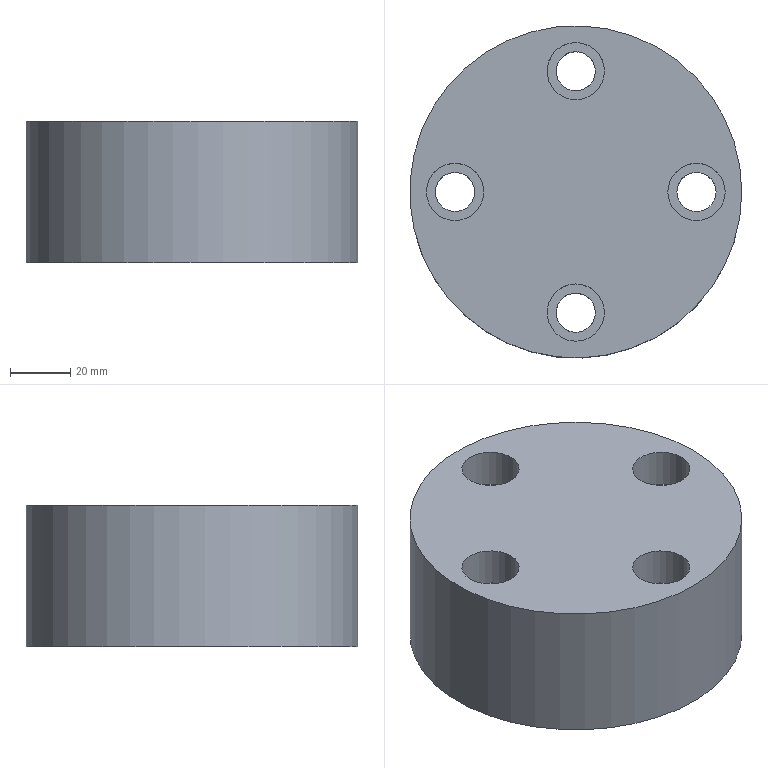NC program | NX | posted with a generic post | part box 110 x 110 x 47 mm
Whole program:
N10 G17 G21 G94 G90
(DRILLING , TOOL : ZXZ)
N12 T01 M6
N14 G54
N16 G17 G0 G90 X0. Y40. S3500 M3
N18 G43 Z30. H1
N20 G94 G81 G98 Z-1. F250. R3.
N22 X-40. Y0.
N24 X0. Y-40.
N26 X40. Y0.
N28 G80
N30 G0 X40. Y0. Z30.
N32 M5
(DRILLING_COPY_COPY , TOOL : 13.0ZT)
N34 T03 M6
N36 G54
N38 G17 G0 G90 X0. Y40. S500 M3
N40 G43 Z30. H3
N42 G94 G83 G98 Z-52.406 F150. Q3. R3.
N44 X-40. Y0.
N46 X0. Y-40.
N48 X40. Y0.
N50 G80
N52 G0 X40. Y0. Z30.
N54 M5
(HOLE_MILLING , TOOL : D10)
N56 T10 M6
N58 G54
N60 G17 G0 G90 X0. Y40. S3000 M3
N62 G43 Z30. H10
N64 Z0.5
N66 G94 G3 X2.25 Y37.75 R2.25 F2200.
N68 X4.5 Y40. R2.25
N70 X4.5 Y40. Z0.28 I-4.5 J0.
N72 X4.5 Y40. Z0.06 I-4.5 J0.
N74 X4.5 Y40. Z-0.16 I-4.5 J0.
N76 X4.5 Y40. Z-0.38 I-4.5 J0.
N78 X4.5 Y40. Z-0.6 I-4.5 J0.
N80 X4.5 Y40. Z-0.82 I-4.5 J0.
N82 X4.5 Y40. Z-1.04 I-4.5 J0.
N84 X4.5 Y40. Z-1.26 I-4.5 J0.
N86 X4.5 Y40. Z-1.48 I-4.5 J0.
N88 X4.5 Y40. Z-1.7 I-4.5 J0.
N90 X4.5 Y40. Z-1.92 I-4.5 J0.
N92 X4.5 Y40. Z-2.14 I-4.5 J0.
N94 X4.5 Y40. Z-2.36 I-4.5 J0.
N96 X4.5 Y40. Z-2.58 I-4.5 J0.
N98 X4.5 Y40. Z-2.8 I-4.5 J0.
N100 X4.5 Y40. Z-3.02 I-4.5 J0.
N102 X4.5 Y40. Z-3.24 I-4.5 J0.
N104 X4.5 Y40. Z-3.46 I-4.5 J0.
N106 X4.5 Y40. Z-3.68 I-4.5 J0.
N108 X4.5 Y40. Z-3.9 I-4.5 J0.
N110 X4.5 Y40. Z-4.12 I-4.5 J0.
N112 X4.5 Y40. Z-4.34 I-4.5 J0.
N114 X4.5 Y40. Z-4.56 I-4.5 J0.
N116 X4.5 Y40. Z-4.78 I-4.5 J0.
N118 X4.5 Y40. Z-5. I-4.5 J0.
N120 X4.5 Y40. Z-5.22 I-4.5 J0.
N122 X4.5 Y40. Z-5.44 I-4.5 J0.
N124 X4.5 Y40. Z-5.66 I-4.5 J0.
N126 X4.5 Y40. Z-5.88 I-4.5 J0.
N128 X4.5 Y40. Z-6.1 I-4.5 J0.
N130 X4.5 Y40. Z-6.32 I-4.5 J0.
N132 X4.5 Y40. Z-6.54 I-4.5 J0.
N134 X4.5 Y40. Z-6.76 I-4.5 J0.
N136 X4.5 Y40. Z-6.98 I-4.5 J0.
N138 X4.5 Y40. Z-7.2 I-4.5 J0.
N140 X4.5 Y40. Z-7.42 I-4.5 J0.
N142 X4.5 Y40. Z-7.64 I-4.5 J0.
N144 X4.5 Y40. Z-7.86 I-4.5 J0.
N146 X4.5 Y40. Z-8.08 I-4.5 J0.
N148 X4.5 Y40. Z-8.3 I-4.5 J0.
N150 X4.5 Y40. Z-8.52 I-4.5 J0.
N152 X4.5 Y40. Z-8.74 I-4.5 J0.
N154 X4.5 Y40. Z-8.96 I-4.5 J0.
N156 X4.5 Y40. Z-9.18 I-4.5 J0.
N158 X4.5 Y40. Z-9.4 I-4.5 J0.
N160 X4.5 Y40. Z-9.62 I-4.5 J0.
N162 X4.5 Y40. Z-9.84 I-4.5 J0.
N164 X4.5 Y40. Z-10.06 I-4.5 J0.
N166 X4.5 Y40. Z-10.28 I-4.5 J0.
N168 X4.5 Y40. Z-10.5 I-4.5 J0.
N170 X4.5 Y40. Z-10.72 I-4.5 J0.
N172 X4.5 Y40. Z-10.94 I-4.5 J0.
N174 X4.5 Y40. Z-11.16 I-4.5 J0.
N176 X4.5 Y40. Z-11.38 I-4.5 J0.
N178 X4.5 Y40. Z-11.6 I-4.5 J0.
N180 X4.5 Y40. Z-11.82 I-4.5 J0.
N182 X4.5 Y40. Z-12.04 I-4.5 J0.
N184 X4.5 Y40. Z-12.26 I-4.5 J0.
N186 X4.5 Y40. Z-12.48 I-4.5 J0.
N188 X4.5 Y40. Z-12.7 I-4.5 J0.
N190 X4.5 Y40. Z-12.92 I-4.5 J0.
N192 X-2.947 Y43.401 Z-13. R4.5
N194 X-3.401 Y37.053 R4.5
N196 X-2.947 Y43.401 R-4.5
N198 X-3.174 Y40.227 R2.25
N200 X0. Y40. R2.25
N202 G0 Z30.
N204 X-40. Y0.
N206 Z0.5
N208 G3 X-37.75 Y-2.25 R2.25
N210 X-35.5 Y0. R2.25
N212 X-35.5 Y0. Z0.28 I-4.5 J0.
N214 X-35.5 Y0. Z0.06 I-4.5 J0.
N216 X-35.5 Y0. Z-0.16 I-4.5 J0.
N218 X-35.5 Y0. Z-0.38 I-4.5 J0.
N220 X-35.5 Y0. Z-0.6 I-4.5 J0.
N222 X-35.5 Y0. Z-0.82 I-4.5 J0.
N224 X-35.5 Y0. Z-1.04 I-4.5 J0.
N226 X-35.5 Y0. Z-1.26 I-4.5 J0.
N228 X-35.5 Y0. Z-1.48 I-4.5 J0.
N230 X-35.5 Y0. Z-1.7 I-4.5 J0.
N232 X-35.5 Y0. Z-1.92 I-4.5 J0.
N234 X-35.5 Y0. Z-2.14 I-4.5 J0.
N236 X-35.5 Y0. Z-2.36 I-4.5 J0.
N238 X-35.5 Y0. Z-2.58 I-4.5 J0.
N240 X-35.5 Y0. Z-2.8 I-4.5 J0.
N242 X-35.5 Y0. Z-3.02 I-4.5 J0.
N244 X-35.5 Y0. Z-3.24 I-4.5 J0.
N246 X-35.5 Y0. Z-3.46 I-4.5 J0.
N248 X-35.5 Y0. Z-3.68 I-4.5 J0.
N250 X-35.5 Y0. Z-3.9 I-4.5 J0.
N252 X-35.5 Y0. Z-4.12 I-4.5 J0.
N254 X-35.5 Y0. Z-4.34 I-4.5 J0.
N256 X-35.5 Y0. Z-4.56 I-4.5 J0.
N258 X-35.5 Y0. Z-4.78 I-4.5 J0.
N260 X-35.5 Y0. Z-5. I-4.5 J0.
N262 X-35.5 Y0. Z-5.22 I-4.5 J0.
N264 X-35.5 Y0. Z-5.44 I-4.5 J0.
N266 X-35.5 Y0. Z-5.66 I-4.5 J0.
N268 X-35.5 Y0. Z-5.88 I-4.5 J0.
N270 X-35.5 Y0. Z-6.1 I-4.5 J0.
N272 X-35.5 Y0. Z-6.32 I-4.5 J0.
N274 X-35.5 Y0. Z-6.54 I-4.5 J0.
N276 X-35.5 Y0. Z-6.76 I-4.5 J0.
N278 X-35.5 Y0. Z-6.98 I-4.5 J0.
N280 X-35.5 Y0. Z-7.2 I-4.5 J0.
N282 X-35.5 Y0. Z-7.42 I-4.5 J0.
N284 X-35.5 Y0. Z-7.64 I-4.5 J0.
N286 X-35.5 Y0. Z-7.86 I-4.5 J0.
N288 X-35.5 Y0. Z-8.08 I-4.5 J0.
N290 X-35.5 Y0. Z-8.3 I-4.5 J0.
N292 X-35.5 Y0. Z-8.52 I-4.5 J0.
N294 X-35.5 Y0. Z-8.74 I-4.5 J0.
N296 X-35.5 Y0. Z-8.96 I-4.5 J0.
N298 X-35.5 Y0. Z-9.18 I-4.5 J0.
N300 X-35.5 Y0. Z-9.4 I-4.5 J0.
N302 X-35.5 Y0. Z-9.62 I-4.5 J0.
N304 X-35.5 Y0. Z-9.84 I-4.5 J0.
N306 X-35.5 Y0. Z-10.06 I-4.5 J0.
N308 X-35.5 Y0. Z-10.28 I-4.5 J0.
N310 X-35.5 Y0. Z-10.5 I-4.5 J0.
N312 X-35.5 Y0. Z-10.72 I-4.5 J0.
N314 X-35.5 Y0. Z-10.94 I-4.5 J0.
N316 X-35.5 Y0. Z-11.16 I-4.5 J0.
N318 X-35.5 Y0. Z-11.38 I-4.5 J0.
N320 X-35.5 Y0. Z-11.6 I-4.5 J0.
N322 X-35.5 Y0. Z-11.82 I-4.5 J0.
N324 X-35.5 Y0. Z-12.04 I-4.5 J0.
N326 X-35.5 Y0. Z-12.26 I-4.5 J0.
N328 X-35.5 Y0. Z-12.48 I-4.5 J0.
N330 X-35.5 Y0. Z-12.7 I-4.5 J0.
N332 X-35.5 Y0. Z-12.92 I-4.5 J0.
N334 X-42.947 Y3.401 Z-13. R4.5
N336 X-43.401 Y-2.947 R4.5
N338 X-42.947 Y3.401 R-4.5
N340 X-43.174 Y0.227 R2.25
N342 X-40. Y0. R2.25
N344 G0 Z30.
N346 X0. Y-40.
N348 Z0.5
N350 G3 X2.25 Y-42.25 R2.25
N352 X4.5 Y-40. R2.25
N354 X4.5 Y-40. Z0.28 I-4.5 J0.
N356 X4.5 Y-40. Z0.06 I-4.5 J0.
N358 X4.5 Y-40. Z-0.16 I-4.5 J0.
N360 X4.5 Y-40. Z-0.38 I-4.5 J0.
N362 X4.5 Y-40. Z-0.6 I-4.5 J0.
N364 X4.5 Y-40. Z-0.82 I-4.5 J0.
N366 X4.5 Y-40. Z-1.04 I-4.5 J0.
N368 X4.5 Y-40. Z-1.26 I-4.5 J0.
N370 X4.5 Y-40. Z-1.48 I-4.5 J0.
N372 X4.5 Y-40. Z-1.7 I-4.5 J0.
N374 X4.5 Y-40. Z-1.92 I-4.5 J0.
N376 X4.5 Y-40. Z-2.14 I-4.5 J0.
N378 X4.5 Y-40. Z-2.36 I-4.5 J0.
N380 X4.5 Y-40. Z-2.58 I-4.5 J0.
N382 X4.5 Y-40. Z-2.8 I-4.5 J0.
N384 X4.5 Y-40. Z-3.02 I-4.5 J0.
N386 X4.5 Y-40. Z-3.24 I-4.5 J0.
N388 X4.5 Y-40. Z-3.46 I-4.5 J0.
N390 X4.5 Y-40. Z-3.68 I-4.5 J0.
N392 X4.5 Y-40. Z-3.9 I-4.5 J0.
N394 X4.5 Y-40. Z-4.12 I-4.5 J0.
N396 X4.5 Y-40. Z-4.34 I-4.5 J0.
N398 X4.5 Y-40. Z-4.56 I-4.5 J0.
N400 X4.5 Y-40. Z-4.78 I-4.5 J0.
N402 X4.5 Y-40. Z-5. I-4.5 J0.
N404 X4.5 Y-40. Z-5.22 I-4.5 J0.
N406 X4.5 Y-40. Z-5.44 I-4.5 J0.
N408 X4.5 Y-40. Z-5.66 I-4.5 J0.
N410 X4.5 Y-40. Z-5.88 I-4.5 J0.
N412 X4.5 Y-40. Z-6.1 I-4.5 J0.
N414 X4.5 Y-40. Z-6.32 I-4.5 J0.
N416 X4.5 Y-40. Z-6.54 I-4.5 J0.
N418 X4.5 Y-40. Z-6.76 I-4.5 J0.
N420 X4.5 Y-40. Z-6.98 I-4.5 J0.
N422 X4.5 Y-40. Z-7.2 I-4.5 J0.
N424 X4.5 Y-40. Z-7.42 I-4.5 J0.
N426 X4.5 Y-40. Z-7.64 I-4.5 J0.
N428 X4.5 Y-40. Z-7.86 I-4.5 J0.
N430 X4.5 Y-40. Z-8.08 I-4.5 J0.
N432 X4.5 Y-40. Z-8.3 I-4.5 J0.
N434 X4.5 Y-40. Z-8.52 I-4.5 J0.
N436 X4.5 Y-40. Z-8.74 I-4.5 J0.
N438 X4.5 Y-40. Z-8.96 I-4.5 J0.
N440 X4.5 Y-40. Z-9.18 I-4.5 J0.
N442 X4.5 Y-40. Z-9.4 I-4.5 J0.
N444 X4.5 Y-40. Z-9.62 I-4.5 J0.
N446 X4.5 Y-40. Z-9.84 I-4.5 J0.
N448 X4.5 Y-40. Z-10.06 I-4.5 J0.
N450 X4.5 Y-40. Z-10.28 I-4.5 J0.
N452 X4.5 Y-40. Z-10.5 I-4.5 J0.
N454 X4.5 Y-40. Z-10.72 I-4.5 J0.
N456 X4.5 Y-40. Z-10.94 I-4.5 J0.
N458 X4.5 Y-40. Z-11.16 I-4.5 J0.
N460 X4.5 Y-40. Z-11.38 I-4.5 J0.
N462 X4.5 Y-40. Z-11.6 I-4.5 J0.
N464 X4.5 Y-40. Z-11.82 I-4.5 J0.
N466 X4.5 Y-40. Z-12.04 I-4.5 J0.
N468 X4.5 Y-40. Z-12.26 I-4.5 J0.
N470 X4.5 Y-40. Z-12.48 I-4.5 J0.
N472 X4.5 Y-40. Z-12.7 I-4.5 J0.
N474 X4.5 Y-40. Z-12.92 I-4.5 J0.
N476 X-2.947 Y-36.599 Z-13. R4.5
N478 X-3.401 Y-42.947 R4.5
N480 X-2.947 Y-36.599 R-4.5
N482 X-3.174 Y-39.773 R2.25
N484 X0. Y-40. R2.25
N486 G0 Z30.
N488 X40. Y0.
N490 Z0.5
N492 G3 X42.25 Y-2.25 R2.25
N494 X44.5 Y0. R2.25
N496 X44.5 Y0. Z0.28 I-4.5 J0.
N498 X44.5 Y0. Z0.06 I-4.5 J0.
N500 X44.5 Y0. Z-0.16 I-4.5 J0.
N502 X44.5 Y0. Z-0.38 I-4.5 J0.
N504 X44.5 Y0. Z-0.6 I-4.5 J0.
N506 X44.5 Y0. Z-0.82 I-4.5 J0.
N508 X44.5 Y0. Z-1.04 I-4.5 J0.
N510 X44.5 Y0. Z-1.26 I-4.5 J0.
N512 X44.5 Y0. Z-1.48 I-4.5 J0.
N514 X44.5 Y0. Z-1.7 I-4.5 J0.
N516 X44.5 Y0. Z-1.92 I-4.5 J0.
N518 X44.5 Y0. Z-2.14 I-4.5 J0.
N520 X44.5 Y0. Z-2.36 I-4.5 J0.
N522 X44.5 Y0. Z-2.58 I-4.5 J0.
N524 X44.5 Y0. Z-2.8 I-4.5 J0.
N526 X44.5 Y0. Z-3.02 I-4.5 J0.
N528 X44.5 Y0. Z-3.24 I-4.5 J0.
N530 X44.5 Y0. Z-3.46 I-4.5 J0.
N532 X44.5 Y0. Z-3.68 I-4.5 J0.
N534 X44.5 Y0. Z-3.9 I-4.5 J0.
N536 X44.5 Y0. Z-4.12 I-4.5 J0.
N538 X44.5 Y0. Z-4.34 I-4.5 J0.
N540 X44.5 Y0. Z-4.56 I-4.5 J0.
N542 X44.5 Y0. Z-4.78 I-4.5 J0.
N544 X44.5 Y0. Z-5. I-4.5 J0.
N546 X44.5 Y0. Z-5.22 I-4.5 J0.
N548 X44.5 Y0. Z-5.44 I-4.5 J0.
N550 X44.5 Y0. Z-5.66 I-4.5 J0.
N552 X44.5 Y0. Z-5.88 I-4.5 J0.
N554 X44.5 Y0. Z-6.1 I-4.5 J0.
N556 X44.5 Y0. Z-6.32 I-4.5 J0.
N558 X44.5 Y0. Z-6.54 I-4.5 J0.
N560 X44.5 Y0. Z-6.76 I-4.5 J0.
N562 X44.5 Y0. Z-6.98 I-4.5 J0.
N564 X44.5 Y0. Z-7.2 I-4.5 J0.
N566 X44.5 Y0. Z-7.42 I-4.5 J0.
N568 X44.5 Y0. Z-7.64 I-4.5 J0.
N570 X44.5 Y0. Z-7.86 I-4.5 J0.
N572 X44.5 Y0. Z-8.08 I-4.5 J0.
N574 X44.5 Y0. Z-8.3 I-4.5 J0.
N576 X44.5 Y0. Z-8.52 I-4.5 J0.
N578 X44.5 Y0. Z-8.74 I-4.5 J0.
N580 X44.5 Y0. Z-8.96 I-4.5 J0.
N582 X44.5 Y0. Z-9.18 I-4.5 J0.
N584 X44.5 Y0. Z-9.4 I-4.5 J0.
N586 X44.5 Y0. Z-9.62 I-4.5 J0.
N588 X44.5 Y0. Z-9.84 I-4.5 J0.
N590 X44.5 Y0. Z-10.06 I-4.5 J0.
N592 X44.5 Y0. Z-10.28 I-4.5 J0.
N594 X44.5 Y0. Z-10.5 I-4.5 J0.
N596 X44.5 Y0. Z-10.72 I-4.5 J0.
N598 X44.5 Y0. Z-10.94 I-4.5 J0.
N600 X44.5 Y0. Z-11.16 I-4.5 J0.
N602 X44.5 Y0. Z-11.38 I-4.5 J0.
N604 X44.5 Y0. Z-11.6 I-4.5 J0.
N606 X44.5 Y0. Z-11.82 I-4.5 J0.
N608 X44.5 Y0. Z-12.04 I-4.5 J0.
N610 X44.5 Y0. Z-12.26 I-4.5 J0.
N612 X44.5 Y0. Z-12.48 I-4.5 J0.
N614 X44.5 Y0. Z-12.7 I-4.5 J0.
N616 X44.5 Y0. Z-12.92 I-4.5 J0.
N618 X37.053 Y3.401 Z-13. R4.5
N620 X36.599 Y-2.947 R4.5
N622 X37.053 Y3.401 R-4.5
N624 X36.826 Y0.227 R2.25
N626 X40. Y0. R2.25
N628 G0 Z30.
N630 M5
(PLANAR_MILL , TOOL : D6A45)
N632 T07 M6
N634 G54
N636 G17 G0 G90 X-7.219 Y41.625 S7500 M3
N638 G43 Z30. H7
N640 Z2.
N642 G94 G1 Z-1. F1250.
N644 X-8.243 Y40.766
N646 G3 X-8.6 Y40. R1.
N648 X0. Y31.4 R8.6
N650 X-8.6 Y40. R-8.6
N652 X-8.243 Y39.234 R1.
N654 G1 X-7.219 Y38.375
N656 Z2.
N658 G0 Z30.
N660 X-32.781 Y-1.625
N662 Z2.
N664 G1 Z-1.
N666 X-31.757 Y-0.766
N668 G3 X-31.4 Y0. R1.
N670 X-40. Y8.6 R8.6
N672 X-31.4 Y0. R-8.6
N674 X-31.757 Y0.766 R1.
N676 G1 X-32.781 Y1.625
N678 Z2.
N680 G0 Z30.
N682 X-7.219 Y-38.375
N684 Z2.
N686 G1 Z-1.
N688 X-8.243 Y-39.234
N690 G3 X-8.6 Y-40. R1.
N692 X0. Y-48.6 R8.6
N694 X-8.6 Y-40. R-8.6
N696 X-8.243 Y-40.766 R1.
N698 G1 X-7.219 Y-41.625
N700 Z2.
N702 G0 Z30.
N704 X32.781 Y1.625
N706 Z2.
N708 G1 Z-1.
N710 X31.757 Y0.766
N712 G3 X31.4 Y0. R1.
N714 X40. Y-8.6 R8.6
N716 X31.4 Y0. R-8.6
N718 X31.757 Y-0.766 R1.
N720 G1 X32.781 Y-1.625
N722 Z2.
N724 G0 Z30.
N726 M5
N728 M2